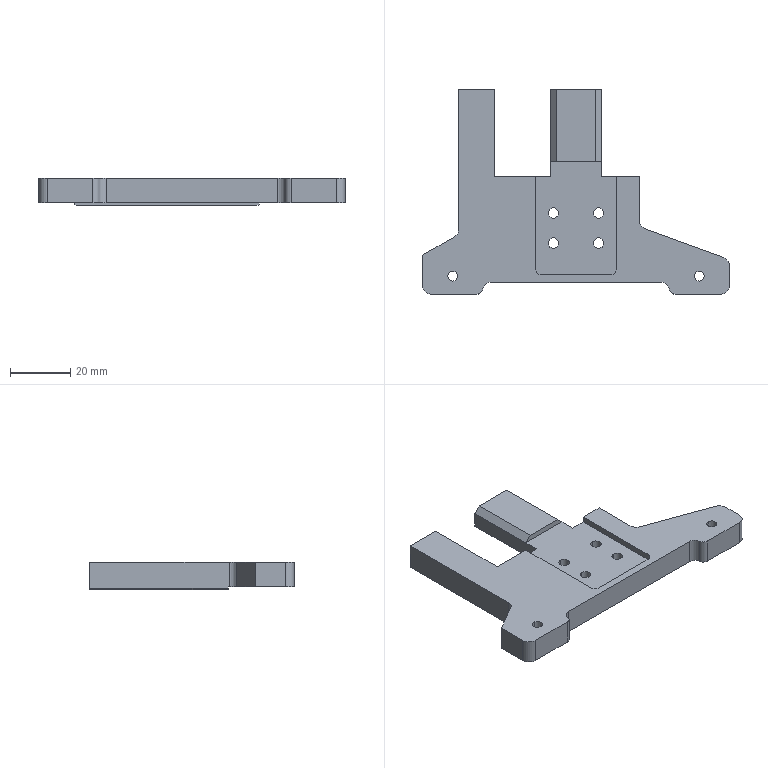CAM job | NX | 3-axis milling, drilling | part box 102 x 68 x 9.2 mm | stock box 111 x 77 x 10.2 mm
Tools:
number,name,description,diameter,corner_radius,flute_length,length,flutes
1,D63,Milling Tool-5 Parameters,63.0,0.0,50.0,75.0,2
7,D6A45,Milling Tool-5 Parameters,6.0,0.0,3.0,3.0,2
13,3.4ZT,Drilling Tool,3.3,0.0,35.0,50.0,2
12,M4,Milling Tool-5 Parameters,3.3,0.0,30.0,30.0,4
15,3.5ZT,Drilling Tool,3.5,0.0,35.0,50.0,2
10,D10,Milling Tool-5 Parameters,10.0,0.0,50.0,75.0,2
4,D4,Milling Tool-5 Parameters,4.0,0.0,50.0,75.0,2
Operations:
program,operation,operation_type,tool,method,geometry_group,spindle_rpm,surface_speed,feed_per_tooth,feed_cut,feed_plunge,cut_length_mm,path_length_mm,cut_time_min,machine_time_min
1-12-72-106,FLOOR_WALL,VolumeBased25DMillingOperation,D63,METHOD,A,6500.0,1286.0,0.0962,1250.0,100.0,585.797,605.797,0.4686,0.4706
1-12-72-106,DRILLING_COPY_1,Operation,D6A45,METHOD,A,3000.0,56.0,0.0333,200.0,0.0,30.6,243.152,0.153,0.1743
1-12-72-106,DRILLING_COPY_1_COPY_COPY_COPY_COPY,Operation,3.4ZT,METHOD,A,2000.0,20.0,0.0375,150.0,0.0,27.983,201.02,0.1866,0.2039
1-12-72-106,DRILLING_COPY_1_COPY_COPY_COPY_COPY_1,Operation,M4,METHOD,A,200.0,2.0,0.0009,0.7,0.0,15.0,175.055,21.429,21.445
1-12-72-106,DRILLING_COPY_1_COPY_COPY_COPY_COPY_COPY,Operation,3.5ZT,METHOD,A,2000.0,20.0,0.0375,150.0,0.0,56.206,220.568,0.3747,0.3911
1-12-72-106,ADAPTIVE_MILLING,CavityMilling,D10,METHOD,A,7000.0,219.0,0.2143,3000.0,1000.0,10974.596,11288.178,3.857,3.889
1-12-72-106,ZLEVEL_PROFILE_COPY_1,ZLevelMilling,D4,METHOD,A,7000.0,87.0,0.1071,1500.0,1000.0,968.033,1985.232,0.6943,0.796
1-12-72-106,FLOOR_WALL_1_COPY_1,VolumeBased25DMillingOperation,D4,METHOD,A,7000.0,87.0,0.0714,1000.0,100.0,574.203,654.01,0.5742,0.5822
1-12-72-106,ZLEVEL_PROFILE_COPY_COPY_1,ZLevelMilling,D4,METHOD,A,7000.0,219.0,0.0714,1000.0,100.0,399.426,439.826,0.3994,0.4035
1-12-72-106,ZLEVEL_PROFILE_COPY_1_COPY_COPY_COPY_COPY_2_COPY,ZLevelMilling,D6A45,METHOD,A,7000.0,131.0,0.0714,1000.0,1000.0,440.641,800.808,0.4406,0.4767
1-12-72-106,ZLEVEL_PROFILE_COPY_1_COPY_COPY_COPY_COPY_2_COPY_COPY,ZLevelMilling,D6A45,METHOD,A,7000.0,131.0,0.0571,800.0,1000.0,73.135,150.651,0.0903,0.098